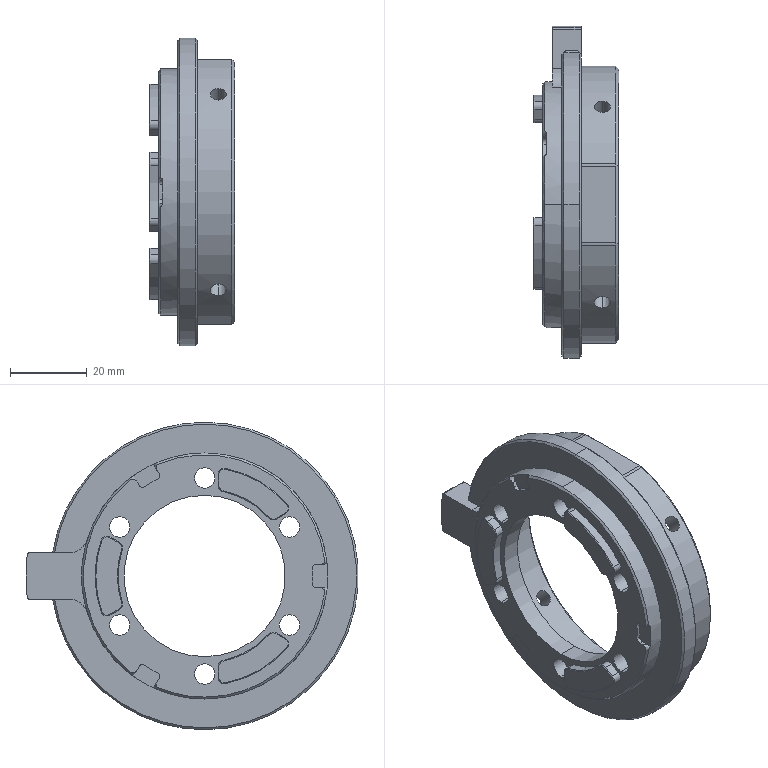NC program | NX | posted with a generic post | part box 22.3 x 86.5 x 80 mm
Lines 1 to 25 of 5076:
N10 G17 G21 G94 G90
(FLOOR_WALL , TOOL : D80)
N12 T19 M6
N14 G54
N16 G17 G0 G90 X-78.124 Y49.087 S6500 M3
N18 G43 Z30. H19
N20 Z3.
N22 G94 G1 Z0. F1500.
N24 X-74.557
N26 X74.55
N28 G2 X84.659 Y28.267 R89.195
N30 X87.825 Y15.918 R89.181
N32 G1 X-87.834
N34 G3 X-89.255 Y1.443 R89.181
N36 G1 Y-1.448
N38 G3 X-87.583 Y-17.25 R89.181
N40 G1 X87.572
N42 X90.628
N44 Z3.
N46 G0 Z30.
N48 M5